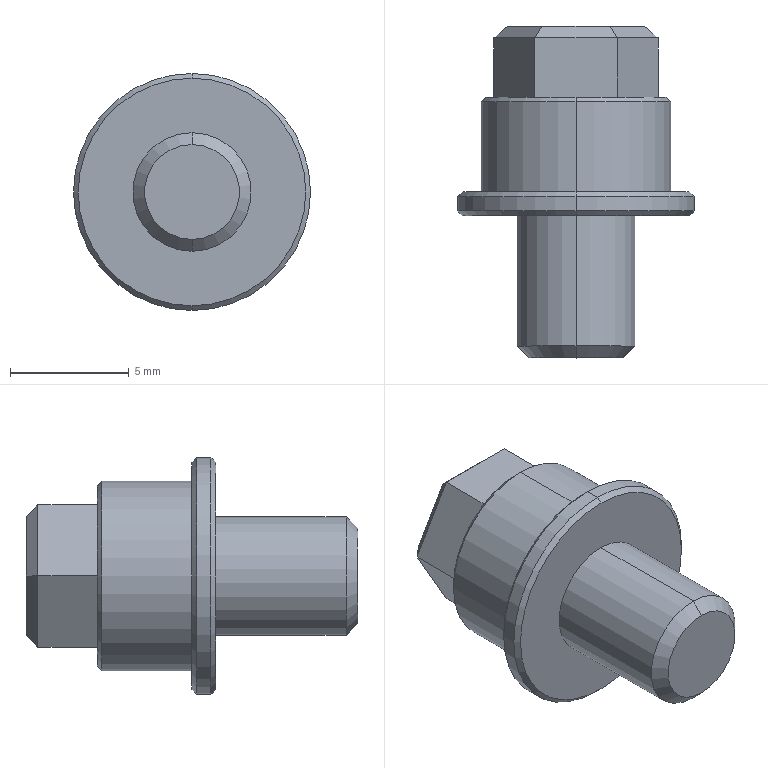Part | SolidWorks | features Chamfer 2, ICE 1, Revolution 1 | 1 solid | 31 faces | box 10 x 14 x 10 mm | volume 484.922 mm3 | plane 17 | cone 8 | cylinder 6 | commonest cylinder face diameters 5 x2 8 x2 10 x2
STEP:
#1=CARTESIAN_POINT('',(0.,7.,4.8));
#2=VERTEX_POINT('',#1);
#3=CARTESIAN_POINT('',(0.,7.,-4.8));
#4=VERTEX_POINT('',#3);
#5=CARTESIAN_POINT('',(0.,7.,0.));
#6=DIRECTION('',(0.,1.,0.));
#7=DIRECTION('',(0.,0.,1.));
#8=AXIS2_PLACEMENT_3D('',#5,#6,#7);
#9=CIRCLE('',#8,4.8);
#10=EDGE_CURVE('',#2,#4,#9,.T.);
#11=ORIENTED_EDGE('',*,*,#10,.F.);
#12=CARTESIAN_POINT('',(0.,6.8,5.));
#13=VERTEX_POINT('',#12);
#14=CARTESIAN_POINT('',(0.,6.8,5.));
#15=DIRECTION('',(0.,-0.7071,0.7071));
#16=VECTOR('',#15,1000.);
#17=LINE('',#14,#16);
#18=EDGE_CURVE('',#2,#13,#17,.T.);
#19=ORIENTED_EDGE('',*,*,#18,.T.);
#20=CARTESIAN_POINT('',(0.,6.8,-5.));
#21=VERTEX_POINT('',#20);
#22=CARTESIAN_POINT('',(0.,6.8,0.));
#23=DIRECTION('',(0.,-1.,0.));
#24=DIRECTION('',(0.,0.,1.));
#25=AXIS2_PLACEMENT_3D('',#22,#23,#24);
#26=CIRCLE('',#25,5.);
#27=EDGE_CURVE('',#21,#13,#26,.T.);
#28=ORIENTED_EDGE('',*,*,#27,.F.);
#29=CARTESIAN_POINT('',(0.,6.8,-5.));
#30=DIRECTION('',(0.,-0.7071,-0.7071));
#31=VECTOR('',#30,1000.);
#32=LINE('',#29,#31);
#33=EDGE_CURVE('',#4,#21,#32,.T.);
#34=ORIENTED_EDGE('',*,*,#33,.F.);
#35=EDGE_LOOP('',(#11,#19,#28,#34));
#36=FACE_OUTER_BOUND('',#35,.T.);
#37=CARTESIAN_POINT('',(0.,6.8,0.));
#38=DIRECTION('',(0.,-1.,0.));
#39=DIRECTION('',(0.,0.,-1.));
#40=AXIS2_PLACEMENT_3D('',#37,#38,#39);
#41=CONICAL_SURFACE('',#40,5.,0.7854);
#42=ADVANCED_FACE('',(#36),#41,.T.);
#43=CARTESIAN_POINT('',(0.,6.,-4.8));
#44=VERTEX_POINT('',#43);
#45=CARTESIAN_POINT('',(0.,6.,4.8));
#46=VERTEX_POINT('',#45);
#47=CARTESIAN_POINT('',(0.,6.,0.));
#48=DIRECTION('',(0.,-1.,0.));
#49=DIRECTION('',(0.,0.,-1.));
#50=AXIS2_PLACEMENT_3D('',#47,#48,#49);
#51=CIRCLE('',#50,4.8);
#52=EDGE_CURVE('',#44,#46,#51,.T.);
#53=ORIENTED_EDGE('',*,*,#52,.F.);
#54=CARTESIAN_POINT('',(0.,6.2,-5.));
#55=VERTEX_POINT('',#54);
#56=CARTESIAN_POINT('',(0.,6.,-4.8));
#57=DIRECTION('',(0.,0.7071,-0.7071));
#58=VECTOR('',#57,1000.);
#59=LINE('',#56,#58);
#60=EDGE_CURVE('',#44,#55,#59,.T.);
#61=ORIENTED_EDGE('',*,*,#60,.T.);
#62=CARTESIAN_POINT('',(0.,6.2,5.));
#63=VERTEX_POINT('',#62);
#64=CARTESIAN_POINT('',(0.,6.2,0.));
#65=DIRECTION('',(0.,1.,0.));
#66=DIRECTION('',(0.,0.,-1.));
#67=AXIS2_PLACEMENT_3D('',#64,#65,#66);
#68=CIRCLE('',#67,5.);
#69=EDGE_CURVE('',#63,#55,#68,.T.);
#70=ORIENTED_EDGE('',*,*,#69,.F.);
#71=CARTESIAN_POINT('',(0.,6.,4.8));
#72=DIRECTION('',(0.,0.7071,0.7071));
#73=VECTOR('',#72,1000.);
#74=LINE('',#71,#73);
#75=EDGE_CURVE('',#46,#63,#74,.T.);
#76=ORIENTED_EDGE('',*,*,#75,.F.);
#77=EDGE_LOOP('',(#53,#61,#70,#76));
#78=FACE_OUTER_BOUND('',#77,.T.);
#79=CARTESIAN_POINT('',(0.,6.,0.));
#80=DIRECTION('',(0.,1.,0.));
#81=DIRECTION('',(0.,0.,1.));
#82=AXIS2_PLACEMENT_3D('',#79,#80,#81);
#83=CONICAL_SURFACE('',#82,4.8,0.7854);
#84=ADVANCED_FACE('',(#78),#83,.T.);
#85=CARTESIAN_POINT('',(0.,11.,3.8));
#86=VERTEX_POINT('',#85);
#87=CARTESIAN_POINT('',(0.,11.,-3.8));
#88=VERTEX_POINT('',#87);
#89=CARTESIAN_POINT('',(0.,11.,0.));
#90=DIRECTION('',(0.,1.,0.));
#91=DIRECTION('',(0.,0.,1.));
#92=AXIS2_PLACEMENT_3D('',#89,#90,#91);
#93=CIRCLE('',#92,3.8);
#94=EDGE_CURVE('',#86,#88,#93,.T.);
#95=ORIENTED_EDGE('',*,*,#94,.F.);
#96=CARTESIAN_POINT('',(0.,10.8,4.));
#97=VERTEX_POINT('',#96);
#98=CARTESIAN_POINT('',(0.,10.8,4.));
#99=DIRECTION('',(0.,-0.7071,0.7071));
#100=VECTOR('',#99,1000.);
#101=LINE('',#98,#100);
#102=EDGE_CURVE('',#86,#97,#101,.T.);
#103=ORIENTED_EDGE('',*,*,#102,.T.);
#104=CARTESIAN_POINT('',(0.,10.8,-4.));
#105=VERTEX_POINT('',#104);
#106=CARTESIAN_POINT('',(0.,10.8,0.));
#107=DIRECTION('',(0.,-1.,0.));
#108=DIRECTION('',(0.,0.,1.));
#109=AXIS2_PLACEMENT_3D('',#106,#107,#108);
#110=CIRCLE('',#109,4.);
#111=EDGE_CURVE('',#105,#97,#110,.T.);
#112=ORIENTED_EDGE('',*,*,#111,.F.);
#113=CARTESIAN_POINT('',(0.,10.8,-4.));
#114=DIRECTION('',(0.,-0.7071,-0.7071));
#115=VECTOR('',#114,1000.);
#116=LINE('',#113,#115);
#117=EDGE_CURVE('',#88,#105,#116,.T.);
#118=ORIENTED_EDGE('',*,*,#117,.F.);
#119=EDGE_LOOP('',(#95,#103,#112,#118));
#120=FACE_OUTER_BOUND('',#119,.T.);
#121=CARTESIAN_POINT('',(0.,10.8,0.));
#122=DIRECTION('',(0.,-1.,0.));
#123=DIRECTION('',(0.,0.,-1.));
#124=AXIS2_PLACEMENT_3D('',#121,#122,#123);
#125=CONICAL_SURFACE('',#124,4.,0.7854);
#126=ADVANCED_FACE('',(#120),#125,.T.);
#127=CARTESIAN_POINT('',(0.,0.,-2.));
#128=VERTEX_POINT('',#127);
#129=CARTESIAN_POINT('',(0.,0.,2.));
#130=VERTEX_POINT('',#129);
#131=CARTESIAN_POINT('',(0.,0.,0.));
#132=DIRECTION('',(0.,-1.,0.));
#133=DIRECTION('',(0.,0.,-1.));
#134=AXIS2_PLACEMENT_3D('',#131,#132,#133);
#135=CIRCLE('',#134,2.);
#136=EDGE_CURVE('',#128,#130,#135,.T.);
#137=ORIENTED_EDGE('',*,*,#136,.F.);
#138=CARTESIAN_POINT('',(0.,0.5,-2.5));
#139=VERTEX_POINT('',#138);
#140=CARTESIAN_POINT('',(0.,0.,-2.));
#141=DIRECTION('',(0.,0.7071,-0.7071));
#142=VECTOR('',#141,1000.);
#143=LINE('',#140,#142);
#144=EDGE_CURVE('',#128,#139,#143,.T.);
#145=ORIENTED_EDGE('',*,*,#144,.T.);
#146=CARTESIAN_POINT('',(0.,0.5,2.5));
#147=VERTEX_POINT('',#146);
#148=CARTESIAN_POINT('',(0.,0.5,0.));
#149=DIRECTION('',(0.,1.,0.));
#150=DIRECTION('',(0.,0.,-1.));
#151=AXIS2_PLACEMENT_3D('',#148,#149,#150);
#152=CIRCLE('',#151,2.5);
#153=EDGE_CURVE('',#147,#139,#152,.T.);
#154=ORIENTED_EDGE('',*,*,#153,.F.);
#155=CARTESIAN_POINT('',(0.,0.,2.));
#156=DIRECTION('',(0.,0.7071,0.7071));
#157=VECTOR('',#156,1000.);
#158=LINE('',#155,#157);
#159=EDGE_CURVE('',#130,#147,#158,.T.);
#160=ORIENTED_EDGE('',*,*,#159,.F.);
#161=EDGE_LOOP('',(#137,#145,#154,#160));
#162=FACE_OUTER_BOUND('',#161,.T.);
#163=CARTESIAN_POINT('',(0.,0.,0.));
#164=DIRECTION('',(0.,1.,0.));
#165=DIRECTION('',(0.,0.,1.));
#166=AXIS2_PLACEMENT_3D('',#163,#164,#165);
#167=CONICAL_SURFACE('',#166,2.,0.7854);
#168=ADVANCED_FACE('',(#162),#167,.T.);
#169=ORIENTED_EDGE('',*,*,#27,.T.);
#170=CARTESIAN_POINT('',(0.,0.,5.));
#171=DIRECTION('',(0.,-1.,0.));
#172=VECTOR('',#171,1000.);
#173=LINE('',#170,#172);
#174=EDGE_CURVE('',#13,#63,#173,.T.);
#175=ORIENTED_EDGE('',*,*,#174,.T.);
#176=ORIENTED_EDGE('',*,*,#69,.T.);
#177=CARTESIAN_POINT('',(0.,0.,-5.));
#178=DIRECTION('',(0.,-1.,0.));
#179=VECTOR('',#178,1000.);
#180=LINE('',#177,#179);
#181=EDGE_CURVE('',#21,#55,#180,.T.);
#182=ORIENTED_EDGE('',*,*,#181,.F.);
#183=EDGE_LOOP('',(#169,#175,#176,#182));
#184=FACE_OUTER_BOUND('',#183,.T.);
#185=CARTESIAN_POINT('',(0.,0.,0.));
#186=DIRECTION('',(0.,-1.,0.));
#187=DIRECTION('',(0.,0.,-1.));
#188=AXIS2_PLACEMENT_3D('',#185,#186,#187);
#189=CYLINDRICAL_SURFACE('',#188,5.);
#190=ADVANCED_FACE('',(#184),#189,.T.);
#191=CARTESIAN_POINT('',(0.,6.,-2.5));
#192=VERTEX_POINT('',#191);
#193=CARTESIAN_POINT('',(0.,6.,2.5));
#194=VERTEX_POINT('',#193);
#195=CARTESIAN_POINT('',(0.,6.,0.));
#196=DIRECTION('',(0.,-1.,0.));
#197=DIRECTION('',(0.,0.,-1.));
#198=AXIS2_PLACEMENT_3D('',#195,#196,#197);
#199=CIRCLE('',#198,2.5);
#200=EDGE_CURVE('',#192,#194,#199,.T.);
#201=ORIENTED_EDGE('',*,*,#200,.T.);
#202=CARTESIAN_POINT('',(0.,0.,2.5));
#203=DIRECTION('',(0.,-1.,0.));
#204=VECTOR('',#203,1000.);
#205=LINE('',#202,#204);
#206=EDGE_CURVE('',#194,#147,#205,.T.);
#207=ORIENTED_EDGE('',*,*,#206,.T.);
#208=ORIENTED_EDGE('',*,*,#153,.T.);
#209=CARTESIAN_POINT('',(0.,0.,-2.5));
#210=DIRECTION('',(0.,-1.,0.));
#211=VECTOR('',#210,1000.);
#212=LINE('',#209,#211);
#213=EDGE_CURVE('',#192,#139,#212,.T.);
#214=ORIENTED_EDGE('',*,*,#213,.F.);
#215=EDGE_LOOP('',(#201,#207,#208,#214));
#216=FACE_OUTER_BOUND('',#215,.T.);
#217=CARTESIAN_POINT('',(0.,0.,0.));
#218=DIRECTION('',(0.,-1.,0.));
#219=DIRECTION('',(0.,0.,-1.));
#220=AXIS2_PLACEMENT_3D('',#217,#218,#219);
#221=CYLINDRICAL_SURFACE('',#220,2.5);
#222=ADVANCED_FACE('',(#216),#221,.T.);
#223=ORIENTED_EDGE('',*,*,#111,.T.);
#224=CARTESIAN_POINT('',(0.,7.,4.));
#225=VERTEX_POINT('',#224);
#226=CARTESIAN_POINT('',(0.,0.,4.));
#227=DIRECTION('',(0.,-1.,0.));
#228=VECTOR('',#227,1000.);
#229=LINE('',#226,#228);
#230=EDGE_CURVE('',#97,#225,#229,.T.);
#231=ORIENTED_EDGE('',*,*,#230,.T.);
#232=CARTESIAN_POINT('',(0.,7.,-4.));
#233=VERTEX_POINT('',#232);
#234=CARTESIAN_POINT('',(0.,7.,0.));
#235=DIRECTION('',(0.,-1.,0.));
#236=DIRECTION('',(0.,0.,-1.));
#237=AXIS2_PLACEMENT_3D('',#234,#235,#236);
#238=CIRCLE('',#237,4.);
#239=EDGE_CURVE('',#233,#225,#238,.T.);
#240=ORIENTED_EDGE('',*,*,#239,.F.);
#241=CARTESIAN_POINT('',(0.,0.,-4.));
#242=DIRECTION('',(0.,-1.,0.));
#243=VECTOR('',#242,1000.);
#244=LINE('',#241,#243);
#245=EDGE_CURVE('',#105,#233,#244,.T.);
#246=ORIENTED_EDGE('',*,*,#245,.F.);
#247=EDGE_LOOP('',(#223,#231,#240,#246));
#248=FACE_OUTER_BOUND('',#247,.T.);
#249=CARTESIAN_POINT('',(0.,0.,0.));
#250=DIRECTION('',(0.,-1.,0.));
#251=DIRECTION('',(0.,0.,-1.));
#252=AXIS2_PLACEMENT_3D('',#249,#250,#251);
#253=CYLINDRICAL_SURFACE('',#252,4.);
#254=ADVANCED_FACE('',(#248),#253,.T.);
#255=ORIENTED_EDGE('',*,*,#230,.F.);
#256=CARTESIAN_POINT('',(0.,10.8,0.));
#257=DIRECTION('',(0.,-1.,0.));
#258=DIRECTION('',(0.,0.,1.));
#259=AXIS2_PLACEMENT_3D('',#256,#257,#258);
#260=CIRCLE('',#259,4.);
#261=EDGE_CURVE('',#97,#105,#260,.T.);
#262=ORIENTED_EDGE('',*,*,#261,.T.);
#263=ORIENTED_EDGE('',*,*,#245,.T.);
#264=CARTESIAN_POINT('',(0.,7.,0.));
#265=DIRECTION('',(0.,-1.,0.));
#266=DIRECTION('',(0.,0.,-1.));
#267=AXIS2_PLACEMENT_3D('',#264,#265,#266);
#268=CIRCLE('',#267,4.);
#269=EDGE_CURVE('',#225,#233,#268,.T.);
#270=ORIENTED_EDGE('',*,*,#269,.F.);
#271=EDGE_LOOP('',(#255,#262,#263,#270));
#272=FACE_OUTER_BOUND('',#271,.T.);
#273=CARTESIAN_POINT('',(0.,0.,0.));
#274=DIRECTION('',(0.,-1.,0.));
#275=DIRECTION('',(0.,0.,-1.));
#276=AXIS2_PLACEMENT_3D('',#273,#274,#275);
#277=CYLINDRICAL_SURFACE('',#276,4.);
#278=ADVANCED_FACE('',(#272),#277,.T.);
#279=CARTESIAN_POINT('',(0.,0.,0.));
#280=DIRECTION('',(0.,-1.,0.));
#281=DIRECTION('',(0.,0.,-1.));
#282=AXIS2_PLACEMENT_3D('',#279,#280,#281);
#283=CIRCLE('',#282,2.);
#284=EDGE_CURVE('',#130,#128,#283,.T.);
#285=ORIENTED_EDGE('',*,*,#284,.T.);
#286=ORIENTED_EDGE('',*,*,#136,.T.);
#287=EDGE_LOOP('',(#285,#286));
#288=FACE_OUTER_BOUND('',#287,.T.);
#289=CARTESIAN_POINT('',(0.,0.,0.));
#290=DIRECTION('',(0.,-1.,0.));
#291=DIRECTION('',(0.,0.,-1.));
#292=AXIS2_PLACEMENT_3D('',#289,#290,#291);
#293=PLANE('',#292);
#294=ADVANCED_FACE('',(#288),#293,.T.);
#295=ORIENTED_EDGE('',*,*,#206,.F.);
#296=CARTESIAN_POINT('',(0.,6.,0.));
#297=DIRECTION('',(0.,-1.,0.));
#298=DIRECTION('',(0.,0.,-1.));
#299=AXIS2_PLACEMENT_3D('',#296,#297,#298);
#300=CIRCLE('',#299,2.5);
#301=EDGE_CURVE('',#194,#192,#300,.T.);
#302=ORIENTED_EDGE('',*,*,#301,.T.);
#303=ORIENTED_EDGE('',*,*,#213,.T.);
#304=CARTESIAN_POINT('',(0.,0.5,0.));
#305=DIRECTION('',(0.,1.,0.));
#306=DIRECTION('',(0.,0.,-1.));
#307=AXIS2_PLACEMENT_3D('',#304,#305,#306);
#308=CIRCLE('',#307,2.5);
#309=EDGE_CURVE('',#139,#147,#308,.T.);
#310=ORIENTED_EDGE('',*,*,#309,.T.);
#311=EDGE_LOOP('',(#295,#302,#303,#310));
#312=FACE_OUTER_BOUND('',#311,.T.);
#313=CARTESIAN_POINT('',(0.,0.,0.));
#314=DIRECTION('',(0.,-1.,0.));
#315=DIRECTION('',(0.,0.,-1.));
#316=AXIS2_PLACEMENT_3D('',#313,#314,#315);
#317=CYLINDRICAL_SURFACE('',#316,2.5);
#318=ADVANCED_FACE('',(#312),#317,.T.);
#319=CARTESIAN_POINT('',(0.,6.,0.));
#320=DIRECTION('',(0.,-1.,0.));
#321=DIRECTION('',(0.,0.,-1.));
#322=AXIS2_PLACEMENT_3D('',#319,#320,#321);
#323=CIRCLE('',#322,4.8);
#324=EDGE_CURVE('',#46,#44,#323,.T.);
#325=ORIENTED_EDGE('',*,*,#324,.T.);
#326=ORIENTED_EDGE('',*,*,#52,.T.);
#327=EDGE_LOOP('',(#325,#326));
#328=FACE_OUTER_BOUND('',#327,.T.);
#329=ORIENTED_EDGE('',*,*,#200,.F.);
#330=ORIENTED_EDGE('',*,*,#301,.F.);
#331=EDGE_LOOP('',(#329,#330));
#332=FACE_BOUND('',#331,.T.);
#333=CARTESIAN_POINT('',(2.5,6.,0.));
#334=DIRECTION('',(0.,-1.,0.));
#335=DIRECTION('',(0.,0.,-1.));
#336=AXIS2_PLACEMENT_3D('',#333,#334,#335);
#337=PLANE('',#336);
#338=ADVANCED_FACE('',(#328,#332),#337,.T.);
#339=ORIENTED_EDGE('',*,*,#174,.F.);
#340=CARTESIAN_POINT('',(0.,6.8,0.));
#341=DIRECTION('',(0.,-1.,0.));
#342=DIRECTION('',(0.,0.,1.));
#343=AXIS2_PLACEMENT_3D('',#340,#341,#342);
#344=CIRCLE('',#343,5.);
#345=EDGE_CURVE('',#13,#21,#344,.T.);
#346=ORIENTED_EDGE('',*,*,#345,.T.);
#347=ORIENTED_EDGE('',*,*,#181,.T.);
#348=CARTESIAN_POINT('',(0.,6.2,0.));
#349=DIRECTION('',(0.,1.,0.));
#350=DIRECTION('',(0.,0.,-1.));
#351=AXIS2_PLACEMENT_3D('',#348,#349,#350);
#352=CIRCLE('',#351,5.);
#353=EDGE_CURVE('',#55,#63,#352,.T.);
#354=ORIENTED_EDGE('',*,*,#353,.T.);
#355=EDGE_LOOP('',(#339,#346,#347,#354));
#356=FACE_OUTER_BOUND('',#355,.T.);
#357=CARTESIAN_POINT('',(0.,0.,0.));
#358=DIRECTION('',(0.,-1.,0.));
#359=DIRECTION('',(0.,0.,-1.));
#360=AXIS2_PLACEMENT_3D('',#357,#358,#359);
#361=CYLINDRICAL_SURFACE('',#360,5.);
#362=ADVANCED_FACE('',(#356),#361,.T.);
#363=CARTESIAN_POINT('',(0.,7.,0.));
#364=DIRECTION('',(0.,1.,0.));
#365=DIRECTION('',(0.,0.,1.));
#366=AXIS2_PLACEMENT_3D('',#363,#364,#365);
#367=CIRCLE('',#366,4.8);
#368=EDGE_CURVE('',#4,#2,#367,.T.);
#369=ORIENTED_EDGE('',*,*,#368,.T.);
#370=ORIENTED_EDGE('',*,*,#10,.T.);
#371=EDGE_LOOP('',(#369,#370));
#372=FACE_OUTER_BOUND('',#371,.T.);
#373=ORIENTED_EDGE('',*,*,#239,.T.);
#374=ORIENTED_EDGE('',*,*,#269,.T.);
#375=EDGE_LOOP('',(#373,#374));
#376=FACE_BOUND('',#375,.T.);
#377=CARTESIAN_POINT('',(5.,7.,0.));
#378=DIRECTION('',(0.,1.,0.));
#379=DIRECTION('',(0.,0.,1.));
#380=AXIS2_PLACEMENT_3D('',#377,#378,#379);
#381=PLANE('',#380);
#382=ADVANCED_FACE('',(#372,#376),#381,.T.);
#383=CARTESIAN_POINT('',(0.,11.,0.));
#384=DIRECTION('',(0.,1.,0.));
#385=DIRECTION('',(0.,0.,1.));
#386=AXIS2_PLACEMENT_3D('',#383,#384,#385);
#387=CIRCLE('',#386,3.8);
#388=EDGE_CURVE('',#88,#86,#387,.T.);
#389=ORIENTED_EDGE('',*,*,#388,.T.);
#390=ORIENTED_EDGE('',*,*,#94,.T.);
#391=EDGE_LOOP('',(#389,#390));
#392=FACE_OUTER_BOUND('',#391,.T.);
#393=CARTESIAN_POINT('',(1.732,11.,3.));
#394=VERTEX_POINT('',#393);
#395=CARTESIAN_POINT('',(3.464,11.,0.));
#396=VERTEX_POINT('',#395);
#397=CARTESIAN_POINT('',(1.732,11.,3.));
#398=DIRECTION('',(0.5,0.,-0.866));
#399=VECTOR('',#398,1000.);
#400=LINE('',#397,#399);
#401=EDGE_CURVE('',#394,#396,#400,.T.);
#402=ORIENTED_EDGE('',*,*,#401,.F.);
#403=CARTESIAN_POINT('',(-1.732,11.,3.));
#404=VERTEX_POINT('',#403);
#405=CARTESIAN_POINT('',(-1.732,11.,3.));
#406=DIRECTION('',(1.,0.,0.));
#407=VECTOR('',#406,1000.);
#408=LINE('',#405,#407);
#409=EDGE_CURVE('',#404,#394,#408,.T.);
#410=ORIENTED_EDGE('',*,*,#409,.F.);
#411=CARTESIAN_POINT('',(-3.464,11.,0.));
#412=VERTEX_POINT('',#411);
#413=CARTESIAN_POINT('',(-3.464,11.,0.));
#414=DIRECTION('',(0.5,0.,0.866));
#415=VECTOR('',#414,1000.);
#416=LINE('',#413,#415);
#417=EDGE_CURVE('',#412,#404,#416,.T.);
#418=ORIENTED_EDGE('',*,*,#417,.F.);
#419=CARTESIAN_POINT('',(-1.732,11.,-3.));
#420=VERTEX_POINT('',#419);
#421=CARTESIAN_POINT('',(-1.732,11.,-3.));
#422=DIRECTION('',(-0.5,0.,0.866));
#423=VECTOR('',#422,1000.);
#424=LINE('',#421,#423);
#425=EDGE_CURVE('',#420,#412,#424,.T.);
#426=ORIENTED_EDGE('',*,*,#425,.F.);
#427=CARTESIAN_POINT('',(1.732,11.,-3.));
#428=VERTEX_POINT('',#427);
#429=CARTESIAN_POINT('',(1.732,11.,-3.));
#430=DIRECTION('',(-1.,0.,0.));
#431=VECTOR('',#430,1000.);
#432=LINE('',#429,#431);
#433=EDGE_CURVE('',#428,#420,#432,.T.);
#434=ORIENTED_EDGE('',*,*,#433,.F.);
#435=CARTESIAN_POINT('',(3.464,11.,0.));
#436=DIRECTION('',(-0.5,0.,-0.866));
#437=VECTOR('',#436,1000.);
#438=LINE('',#435,#437);
#439=EDGE_CURVE('',#396,#428,#438,.T.);
#440=ORIENTED_EDGE('',*,*,#439,.F.);
#441=EDGE_LOOP('',(#402,#410,#418,#426,#434,#440));
#442=FACE_BOUND('',#441,.T.);
#443=CARTESIAN_POINT('',(0.,11.,0.));
#444=DIRECTION('',(0.,1.,0.));
#445=DIRECTION('',(0.,0.,1.));
#446=AXIS2_PLACEMENT_3D('',#443,#444,#445);
#447=PLANE('',#446);
#448=ADVANCED_FACE('',(#392,#442),#447,.T.);
#449=CARTESIAN_POINT('',(1.732,13.5,-3.));
#450=VERTEX_POINT('',#449);
#451=CARTESIAN_POINT('',(1.732,11.,-3.));
#452=DIRECTION('',(0.,1.,0.));
#453=VECTOR('',#452,1000.);
#454=LINE('',#451,#453);
#455=EDGE_CURVE('',#428,#450,#454,.T.);
#456=ORIENTED_EDGE('',*,*,#455,.T.);
#457=CARTESIAN_POINT('',(3.464,13.5,0.));
#458=VERTEX_POINT('',#457);
#459=CARTESIAN_POINT('',(3.464,13.5,0.));
#460=DIRECTION('',(0.5,0.,0.866));
#461=VECTOR('',#460,1000.);
#462=LINE('',#459,#461);
#463=EDGE_CURVE('',#450,#458,#462,.T.);
#464=ORIENTED_EDGE('',*,*,#463,.T.);
#465=CARTESIAN_POINT('',(3.464,11.,0.));
#466=DIRECTION('',(0.,1.,0.));
#467=VECTOR('',#466,1000.);
#468=LINE('',#465,#467);
#469=EDGE_CURVE('',#396,#458,#468,.T.);
#470=ORIENTED_EDGE('',*,*,#469,.F.);
#471=ORIENTED_EDGE('',*,*,#439,.T.);
#472=EDGE_LOOP('',(#456,#464,#470,#471));
#473=FACE_OUTER_BOUND('',#472,.T.);
#474=CARTESIAN_POINT('',(3.464,11.,0.));
#475=DIRECTION('',(0.866,0.,-0.5));
#476=DIRECTION('',(-0.5,0.,-0.866));
#477=AXIS2_PLACEMENT_3D('',#474,#475,#476);
#478=PLANE('',#477);
#479=ADVANCED_FACE('',(#473),#478,.T.);
#480=ORIENTED_EDGE('',*,*,#469,.T.);
#481=CARTESIAN_POINT('',(1.732,13.5,3.));
#482=VERTEX_POINT('',#481);
#483=CARTESIAN_POINT('',(1.732,13.5,3.));
#484=DIRECTION('',(-0.5,0.,0.866));
#485=VECTOR('',#484,1000.);
#486=LINE('',#483,#485);
#487=EDGE_CURVE('',#458,#482,#486,.T.);
#488=ORIENTED_EDGE('',*,*,#487,.T.);
#489=CARTESIAN_POINT('',(1.732,11.,3.));
#490=DIRECTION('',(0.,1.,0.));
#491=VECTOR('',#490,1000.);
#492=LINE('',#489,#491);
#493=EDGE_CURVE('',#394,#482,#492,.T.);
#494=ORIENTED_EDGE('',*,*,#493,.F.);
#495=ORIENTED_EDGE('',*,*,#401,.T.);
#496=EDGE_LOOP('',(#480,#488,#494,#495));
#497=FACE_OUTER_BOUND('',#496,.T.);
#498=CARTESIAN_POINT('',(1.732,11.,3.));
#499=DIRECTION('',(0.866,0.,0.5));
#500=DIRECTION('',(0.5,0.,-0.866));
#501=AXIS2_PLACEMENT_3D('',#498,#499,#500);
#502=PLANE('',#501);
#503=ADVANCED_FACE('',(#497),#502,.T.);
#504=ORIENTED_EDGE('',*,*,#493,.T.);
#505=CARTESIAN_POINT('',(-1.732,13.5,3.));
#506=VERTEX_POINT('',#505);
#507=CARTESIAN_POINT('',(-1.732,13.5,3.));
#508=DIRECTION('',(-1.,0.,0.));
#509=VECTOR('',#508,1000.);
#510=LINE('',#507,#509);
#511=EDGE_CURVE('',#482,#506,#510,.T.);
#512=ORIENTED_EDGE('',*,*,#511,.T.);
#513=CARTESIAN_POINT('',(-1.732,11.,3.));
#514=DIRECTION('',(0.,1.,0.));
#515=VECTOR('',#514,1000.);
#516=LINE('',#513,#515);
#517=EDGE_CURVE('',#404,#506,#516,.T.);
#518=ORIENTED_EDGE('',*,*,#517,.F.);
#519=ORIENTED_EDGE('',*,*,#409,.T.);
#520=EDGE_LOOP('',(#504,#512,#518,#519));
#521=FACE_OUTER_BOUND('',#520,.T.);
#522=CARTESIAN_POINT('',(-1.732,11.,3.));
#523=DIRECTION('',(0.,0.,1.));
#524=DIRECTION('',(1.,0.,0.));
#525=AXIS2_PLACEMENT_3D('',#522,#523,#524);
#526=PLANE('',#525);
#527=ADVANCED_FACE('',(#521),#526,.T.);
#528=ORIENTED_EDGE('',*,*,#517,.T.);
#529=CARTESIAN_POINT('',(-3.464,13.5,0.));
#530=VERTEX_POINT('',#529);
#531=CARTESIAN_POINT('',(-3.464,13.5,0.));
#532=DIRECTION('',(-0.5,0.,-0.866));
#533=VECTOR('',#532,1000.);
#534=LINE('',#531,#533);
#535=EDGE_CURVE('',#506,#530,#534,.T.);
#536=ORIENTED_EDGE('',*,*,#535,.T.);
#537=CARTESIAN_POINT('',(-3.464,11.,0.));
#538=DIRECTION('',(0.,1.,0.));
#539=VECTOR('',#538,1000.);
#540=LINE('',#537,#539);
#541=EDGE_CURVE('',#412,#530,#540,.T.);
#542=ORIENTED_EDGE('',*,*,#541,.F.);
#543=ORIENTED_EDGE('',*,*,#417,.T.);
#544=EDGE_LOOP('',(#528,#536,#542,#543));
#545=FACE_OUTER_BOUND('',#544,.T.);
#546=CARTESIAN_POINT('',(-3.464,11.,0.));
#547=DIRECTION('',(-0.866,0.,0.5));
#548=DIRECTION('',(0.5,0.,0.866));
#549=AXIS2_PLACEMENT_3D('',#546,#547,#548);
#550=PLANE('',#549);
#551=ADVANCED_FACE('',(#545),#550,.T.);
#552=ORIENTED_EDGE('',*,*,#541,.T.);
#553=CARTESIAN_POINT('',(-1.732,13.5,-3.));
#554=VERTEX_POINT('',#553);
#555=CARTESIAN_POINT('',(-1.732,13.5,-3.));
#556=DIRECTION('',(0.5,0.,-0.866));
#557=VECTOR('',#556,1000.);
#558=LINE('',#555,#557);
#559=EDGE_CURVE('',#530,#554,#558,.T.);
#560=ORIENTED_EDGE('',*,*,#559,.T.);
#561=CARTESIAN_POINT('',(-1.732,11.,-3.));
#562=DIRECTION('',(0.,1.,0.));
#563=VECTOR('',#562,1000.);
#564=LINE('',#561,#563);
#565=EDGE_CURVE('',#420,#554,#564,.T.);
#566=ORIENTED_EDGE('',*,*,#565,.F.);
#567=ORIENTED_EDGE('',*,*,#425,.T.);
#568=EDGE_LOOP('',(#552,#560,#566,#567));
#569=FACE_OUTER_BOUND('',#568,.T.);
#570=CARTESIAN_POINT('',(-1.732,11.,-3.));
#571=DIRECTION('',(-0.866,0.,-0.5));
#572=DIRECTION('',(-0.5,0.,0.866));
#573=AXIS2_PLACEMENT_3D('',#570,#571,#572);
#574=PLANE('',#573);
#575=ADVANCED_FACE('',(#569),#574,.T.);
#576=ORIENTED_EDGE('',*,*,#565,.T.);
#577=CARTESIAN_POINT('',(1.732,13.5,-3.));
#578=DIRECTION('',(1.,0.,0.));
#579=VECTOR('',#578,1000.);
#580=LINE('',#577,#579);
#581=EDGE_CURVE('',#554,#450,#580,.T.);
#582=ORIENTED_EDGE('',*,*,#581,.T.);
#583=ORIENTED_EDGE('',*,*,#455,.F.);
#584=ORIENTED_EDGE('',*,*,#433,.T.);
#585=EDGE_LOOP('',(#576,#582,#583,#584));
#586=FACE_OUTER_BOUND('',#585,.T.);
#587=CARTESIAN_POINT('',(1.732,11.,-3.));
#588=DIRECTION('',(0.,0.,-1.));
#589=DIRECTION('',(-1.,0.,0.));
#590=AXIS2_PLACEMENT_3D('',#587,#588,#589);
#591=PLANE('',#590);
#592=ADVANCED_FACE('',(#586),#591,.T.);
#593=CARTESIAN_POINT('',(-2.887,14.,0.));
#594=VERTEX_POINT('',#593);
#595=CARTESIAN_POINT('',(-1.443,14.,2.5));
#596=VERTEX_POINT('',#595);
#597=CARTESIAN_POINT('',(-1.165,14.,2.982));
#598=DIRECTION('',(0.5,0.,0.866));
#599=VECTOR('',#598,1000.);
#600=LINE('',#597,#599);
#601=EDGE_CURVE('',#594,#596,#600,.T.);
#602=ORIENTED_EDGE('',*,*,#601,.T.);
#603=CARTESIAN_POINT('',(1.443,14.,2.5));
#604=VERTEX_POINT('',#603);
#605=CARTESIAN_POINT('',(4.,14.,2.5));
#606=DIRECTION('',(1.,0.,0.));
#607=VECTOR('',#606,1000.);
#608=LINE('',#605,#607);
#609=EDGE_CURVE('',#596,#604,#608,.T.);
#610=ORIENTED_EDGE('',*,*,#609,.T.);
#611=CARTESIAN_POINT('',(2.887,14.,0.));
#612=VERTEX_POINT('',#611);
#613=CARTESIAN_POINT('',(3.165,14.,-0.4821));
#614=DIRECTION('',(0.5,0.,-0.866));
#615=VECTOR('',#614,1000.);
#616=LINE('',#613,#615);
#617=EDGE_CURVE('',#604,#612,#616,.T.);
#618=ORIENTED_EDGE('',*,*,#617,.T.);
#619=CARTESIAN_POINT('',(1.443,14.,-2.5));
#620=VERTEX_POINT('',#619);
#621=CARTESIAN_POINT('',(3.165,14.,0.4821));
#622=DIRECTION('',(-0.5,0.,-0.866));
#623=VECTOR('',#622,1000.);
#624=LINE('',#621,#623);
#625=EDGE_CURVE('',#612,#620,#624,.T.);
#626=ORIENTED_EDGE('',*,*,#625,.T.);
#627=CARTESIAN_POINT('',(-1.443,14.,-2.5));
#628=VERTEX_POINT('',#627);
#629=CARTESIAN_POINT('',(4.,14.,-2.5));
#630=DIRECTION('',(-1.,0.,0.));
#631=VECTOR('',#630,1000.);
#632=LINE('',#629,#631);
#633=EDGE_CURVE('',#620,#628,#632,.T.);
#634=ORIENTED_EDGE('',*,*,#633,.T.);
#635=CARTESIAN_POINT('',(-1.165,14.,-2.982));
#636=DIRECTION('',(-0.5,0.,0.866));
#637=VECTOR('',#636,1000.);
#638=LINE('',#635,#637);
#639=EDGE_CURVE('',#628,#594,#638,.T.);
#640=ORIENTED_EDGE('',*,*,#639,.T.);
#641=EDGE_LOOP('',(#602,#610,#618,#626,#634,#640));
#642=FACE_OUTER_BOUND('',#641,.T.);
#643=CARTESIAN_POINT('',(4.,14.,0.));
#644=DIRECTION('',(0.,1.,0.));
#645=DIRECTION('',(0.,0.,1.));
#646=AXIS2_PLACEMENT_3D('',#643,#644,#645);
#647=PLANE('',#646);
#648=ADVANCED_FACE('',(#642),#647,.T.);
#649=CARTESIAN_POINT('',(0.9515,14.852,-1.648));
#650=DIRECTION('',(-0.378,0.6547,0.6547));
#651=VECTOR('',#650,1000.);
#652=LINE('',#649,#651);
#653=EDGE_CURVE('',#450,#620,#652,.T.);
#654=ORIENTED_EDGE('',*,*,#653,.F.);
#655=ORIENTED_EDGE('',*,*,#581,.F.);
#656=CARTESIAN_POINT('',(-0.6658,15.347,-1.153));
#657=DIRECTION('',(-0.378,-0.6547,-0.6547));
#658=VECTOR('',#657,1000.);
#659=LINE('',#656,#658);
#660=EDGE_CURVE('',#628,#554,#659,.T.);
#661=ORIENTED_EDGE('',*,*,#660,.F.);
#662=ORIENTED_EDGE('',*,*,#633,.F.);
#663=EDGE_LOOP('',(#654,#655,#661,#662));
#664=FACE_OUTER_BOUND('',#663,.T.);
#665=CARTESIAN_POINT('',(4.,14.,-2.5));
#666=DIRECTION('',(0.,-0.7071,0.7071));
#667=DIRECTION('',(-1.,0.,0.));
#668=AXIS2_PLACEMENT_3D('',#665,#666,#667);
#669=PLANE('',#668);
#670=ADVANCED_FACE('',(#664),#669,.F.);
#671=ORIENTED_EDGE('',*,*,#660,.T.);
#672=ORIENTED_EDGE('',*,*,#559,.F.);
#673=CARTESIAN_POINT('',(-1.903,14.852,0.));
#674=DIRECTION('',(-0.7559,-0.6547,0.));
#675=VECTOR('',#674,1000.);
#676=LINE('',#673,#675);
#677=EDGE_CURVE('',#594,#530,#676,.T.);
#678=ORIENTED_EDGE('',*,*,#677,.F.);
#679=ORIENTED_EDGE('',*,*,#639,.F.);
#680=EDGE_LOOP('',(#671,#672,#678,#679));
#681=FACE_OUTER_BOUND('',#680,.T.);
#682=CARTESIAN_POINT('',(-1.165,14.,-2.982));
#683=DIRECTION('',(0.6124,-0.7071,0.3536));
#684=DIRECTION('',(-0.5,0.,0.866));
#685=AXIS2_PLACEMENT_3D('',#682,#683,#684);
#686=PLANE('',#685);
#687=ADVANCED_FACE('',(#681),#686,.F.);
#688=ORIENTED_EDGE('',*,*,#653,.T.);
#689=ORIENTED_EDGE('',*,*,#625,.F.);
#690=CARTESIAN_POINT('',(3.046,13.862,0.));
#691=DIRECTION('',(-0.7559,0.6547,0.));
#692=VECTOR('',#691,1000.);
#693=LINE('',#690,#692);
#694=EDGE_CURVE('',#458,#612,#693,.T.);
#695=ORIENTED_EDGE('',*,*,#694,.F.);
#696=ORIENTED_EDGE('',*,*,#463,.F.);
#697=EDGE_LOOP('',(#688,#689,#695,#696));
#698=FACE_OUTER_BOUND('',#697,.T.);
#699=CARTESIAN_POINT('',(3.165,14.,0.4821));
#700=DIRECTION('',(-0.6124,-0.7071,0.3536));
#701=DIRECTION('',(-0.5,0.,-0.866));
#702=AXIS2_PLACEMENT_3D('',#699,#700,#701);
#703=PLANE('',#702);
#704=ADVANCED_FACE('',(#698),#703,.F.);
#705=ORIENTED_EDGE('',*,*,#677,.T.);
#706=ORIENTED_EDGE('',*,*,#535,.F.);
#707=CARTESIAN_POINT('',(-1.523,13.862,2.638));
#708=DIRECTION('',(-0.378,-0.6547,0.6547));
#709=VECTOR('',#708,1000.);
#710=LINE('',#707,#709);
#711=EDGE_CURVE('',#596,#506,#710,.T.);
#712=ORIENTED_EDGE('',*,*,#711,.F.);
#713=ORIENTED_EDGE('',*,*,#601,.F.);
#714=EDGE_LOOP('',(#705,#706,#712,#713));
#715=FACE_OUTER_BOUND('',#714,.T.);
#716=CARTESIAN_POINT('',(-1.165,14.,2.982));
#717=DIRECTION('',(0.6124,-0.7071,-0.3536));
#718=DIRECTION('',(0.5,0.,0.866));
#719=AXIS2_PLACEMENT_3D('',#716,#717,#718);
#720=PLANE('',#719);
#721=ADVANCED_FACE('',(#715),#720,.F.);
#722=ORIENTED_EDGE('',*,*,#694,.T.);
#723=ORIENTED_EDGE('',*,*,#617,.F.);
#724=CARTESIAN_POINT('',(0.9515,14.852,1.648));
#725=DIRECTION('',(-0.378,0.6547,-0.6547));
#726=VECTOR('',#725,1000.);
#727=LINE('',#724,#726);
#728=EDGE_CURVE('',#482,#604,#727,.T.);
#729=ORIENTED_EDGE('',*,*,#728,.F.);
#730=ORIENTED_EDGE('',*,*,#487,.F.);
#731=EDGE_LOOP('',(#722,#723,#729,#730));
#732=FACE_OUTER_BOUND('',#731,.T.);
#733=CARTESIAN_POINT('',(3.165,14.,-0.4821));
#734=DIRECTION('',(-0.6124,-0.7071,-0.3536));
#735=DIRECTION('',(0.5,0.,-0.866));
#736=AXIS2_PLACEMENT_3D('',#733,#734,#735);
#737=PLANE('',#736);
#738=ADVANCED_FACE('',(#732),#737,.F.);
#739=ORIENTED_EDGE('',*,*,#711,.T.);
#740=ORIENTED_EDGE('',*,*,#511,.F.);
#741=ORIENTED_EDGE('',*,*,#728,.T.);
#742=ORIENTED_EDGE('',*,*,#609,.F.);
#743=EDGE_LOOP('',(#739,#740,#741,#742));
#744=FACE_OUTER_BOUND('',#743,.T.);
#745=CARTESIAN_POINT('',(4.,14.,2.5));
#746=DIRECTION('',(0.,-0.7071,-0.7071));
#747=DIRECTION('',(1.,0.,0.));
#748=AXIS2_PLACEMENT_3D('',#745,#746,#747);
#749=PLANE('',#748);
#750=ADVANCED_FACE('',(#744),#749,.F.);
#751=ORIENTED_EDGE('',*,*,#144,.F.);
#752=ORIENTED_EDGE('',*,*,#284,.F.);
#753=ORIENTED_EDGE('',*,*,#159,.T.);
#754=ORIENTED_EDGE('',*,*,#309,.F.);
#755=EDGE_LOOP('',(#751,#752,#753,#754));
#756=FACE_OUTER_BOUND('',#755,.T.);
#757=CARTESIAN_POINT('',(0.,0.,0.));
#758=DIRECTION('',(0.,1.,0.));
#759=DIRECTION('',(0.,0.,1.));
#760=AXIS2_PLACEMENT_3D('',#757,#758,#759);
#761=CONICAL_SURFACE('',#760,2.,0.7854);
#762=ADVANCED_FACE('',(#756),#761,.T.);
#763=ORIENTED_EDGE('',*,*,#102,.F.);
#764=ORIENTED_EDGE('',*,*,#388,.F.);
#765=ORIENTED_EDGE('',*,*,#117,.T.);
#766=ORIENTED_EDGE('',*,*,#261,.F.);
#767=EDGE_LOOP('',(#763,#764,#765,#766));
#768=FACE_OUTER_BOUND('',#767,.T.);
#769=CARTESIAN_POINT('',(0.,10.8,0.));
#770=DIRECTION('',(0.,-1.,0.));
#771=DIRECTION('',(0.,0.,-1.));
#772=AXIS2_PLACEMENT_3D('',#769,#770,#771);
#773=CONICAL_SURFACE('',#772,4.,0.7854);
#774=ADVANCED_FACE('',(#768),#773,.T.);
#775=ORIENTED_EDGE('',*,*,#60,.F.);
#776=ORIENTED_EDGE('',*,*,#324,.F.);
#777=ORIENTED_EDGE('',*,*,#75,.T.);
#778=ORIENTED_EDGE('',*,*,#353,.F.);
#779=EDGE_LOOP('',(#775,#776,#777,#778));
#780=FACE_OUTER_BOUND('',#779,.T.);
#781=CARTESIAN_POINT('',(0.,6.,0.));
#782=DIRECTION('',(0.,1.,0.));
#783=DIRECTION('',(0.,0.,1.));
#784=AXIS2_PLACEMENT_3D('',#781,#782,#783);
#785=CONICAL_SURFACE('',#784,4.8,0.7854);
#786=ADVANCED_FACE('',(#780),#785,.T.);
#787=ORIENTED_EDGE('',*,*,#18,.F.);
#788=ORIENTED_EDGE('',*,*,#368,.F.);
#789=ORIENTED_EDGE('',*,*,#33,.T.);
#790=ORIENTED_EDGE('',*,*,#345,.F.);
#791=EDGE_LOOP('',(#787,#788,#789,#790));
#792=FACE_OUTER_BOUND('',#791,.T.);
#793=CARTESIAN_POINT('',(0.,6.8,0.));
#794=DIRECTION('',(0.,-1.,0.));
#795=DIRECTION('',(0.,0.,-1.));
#796=AXIS2_PLACEMENT_3D('',#793,#794,#795);
#797=CONICAL_SURFACE('',#796,5.,0.7854);
#798=ADVANCED_FACE('',(#792),#797,.T.);
#799=CLOSED_SHELL('',(#42,#84,#126,#168,#190,#222,#254,#278,#294,#318,#338,#362,#382,#448,#479,#503,#527,#551,#575,#592,#648,#670,#687,#704,#721,#738,#750,#762,#774,#786,#798));
#800=MANIFOLD_SOLID_BREP('',#799);
#801=CARTESIAN_POINT('',(0.,0.,0.));
#802=DIRECTION('',(0.,0.,1.));
#803=DIRECTION('',(1.,0.,0.));
#804=AXIS2_PLACEMENT_3D('',#801,#802,#803);
#805=(LENGTH_UNIT()NAMED_UNIT(*)SI_UNIT(.MILLI.,.METRE.));
#806=UNCERTAINTY_MEASURE_WITH_UNIT(LENGTH_MEASURE(0.00001),#805,'','');
#807=(NAMED_UNIT(*)PLANE_ANGLE_UNIT()SI_UNIT($,.RADIAN.));
#808=(NAMED_UNIT(*)SI_UNIT($,.STERADIAN.)SOLID_ANGLE_UNIT());
#809=(GEOMETRIC_REPRESENTATION_CONTEXT(3)GLOBAL_UNCERTAINTY_ASSIGNED_CONTEXT((#806))GLOBAL_UNIT_ASSIGNED_CONTEXT((#805,#807,#808))REPRESENTATION_CONTEXT('',''));
#810=ADVANCED_BREP_SHAPE_REPRESENTATION('',(#800,#804),#809);